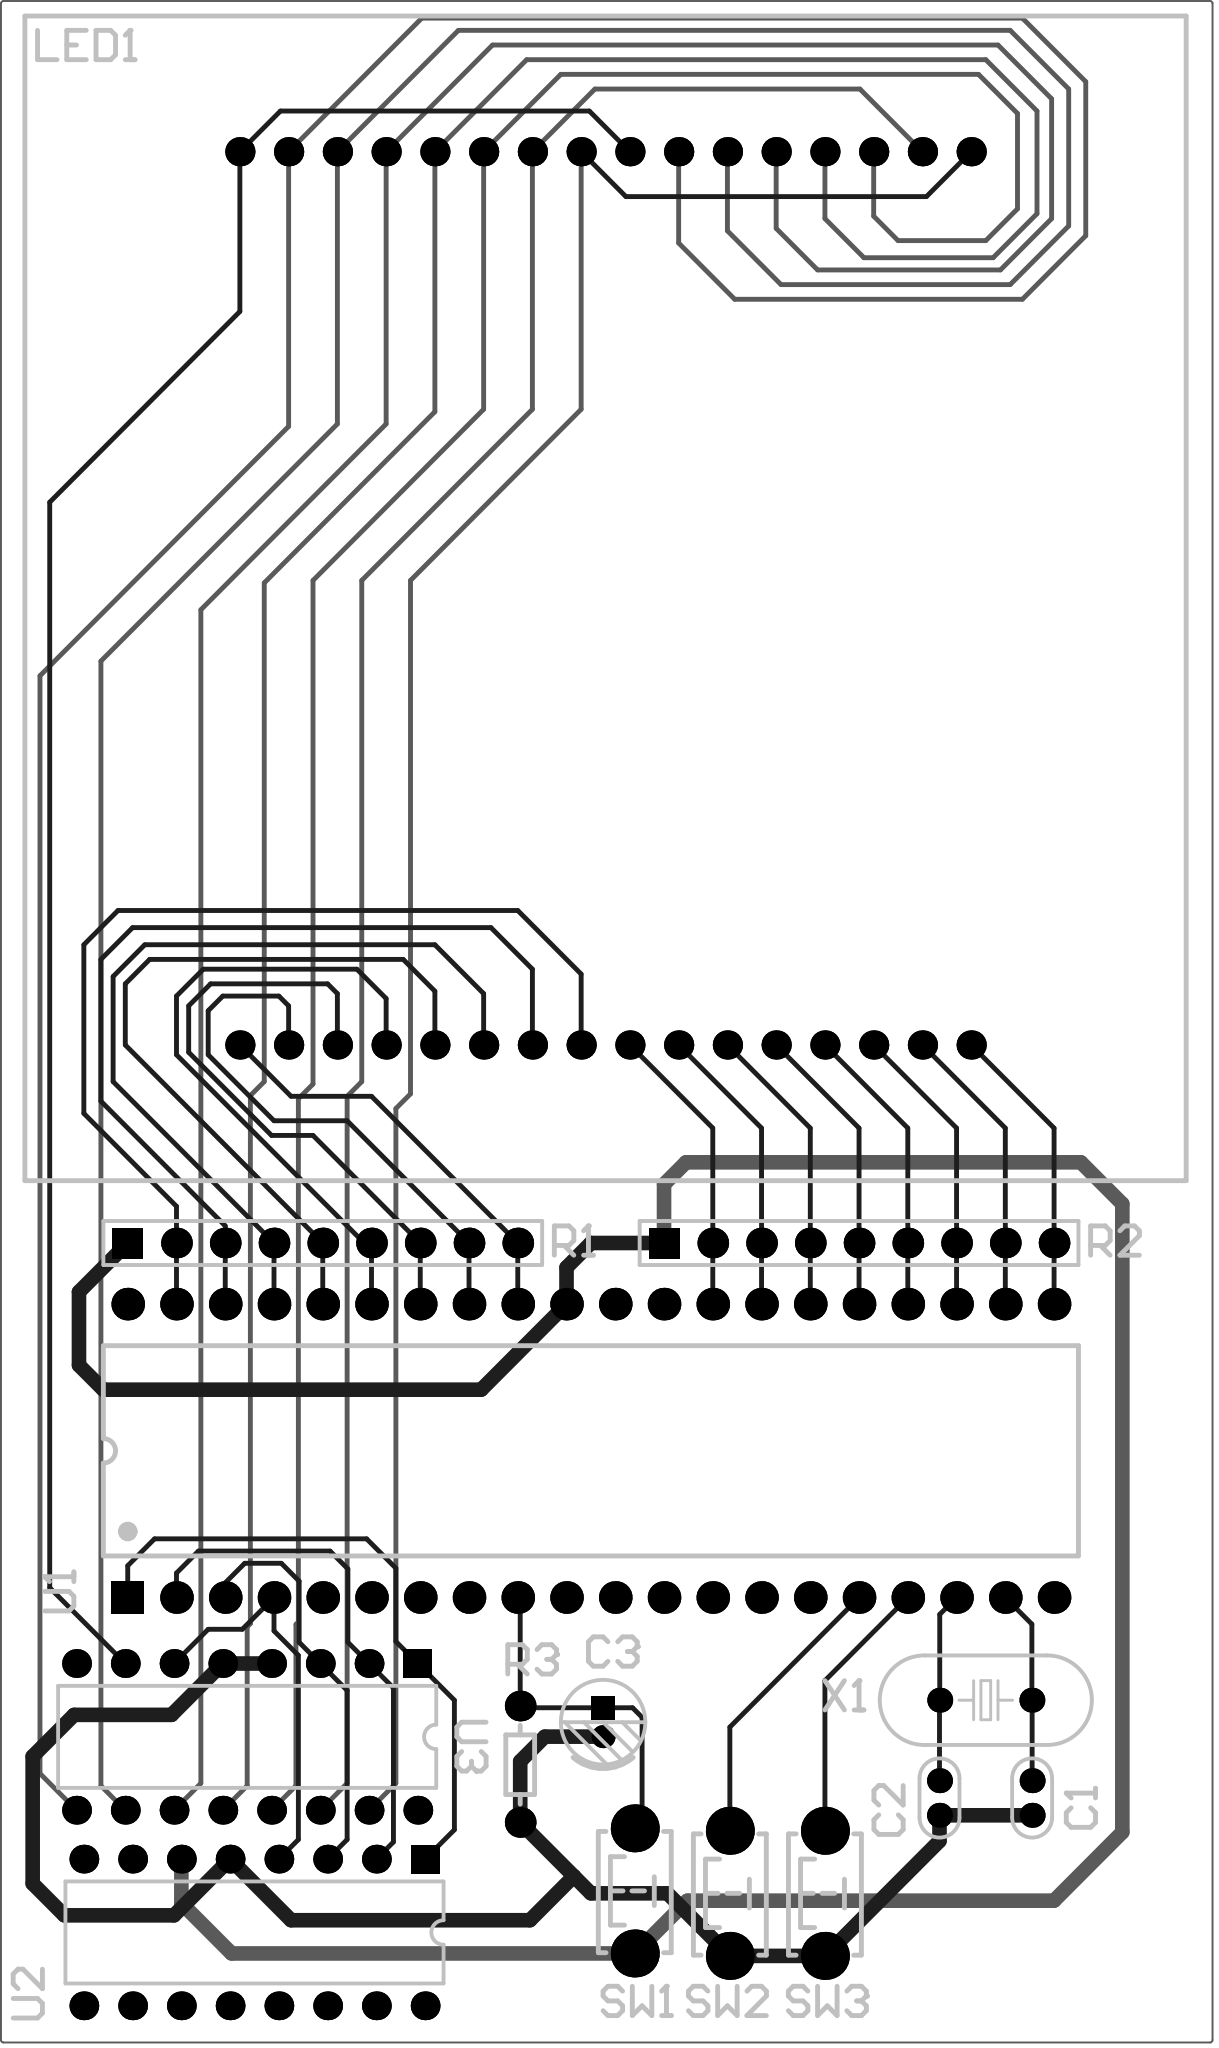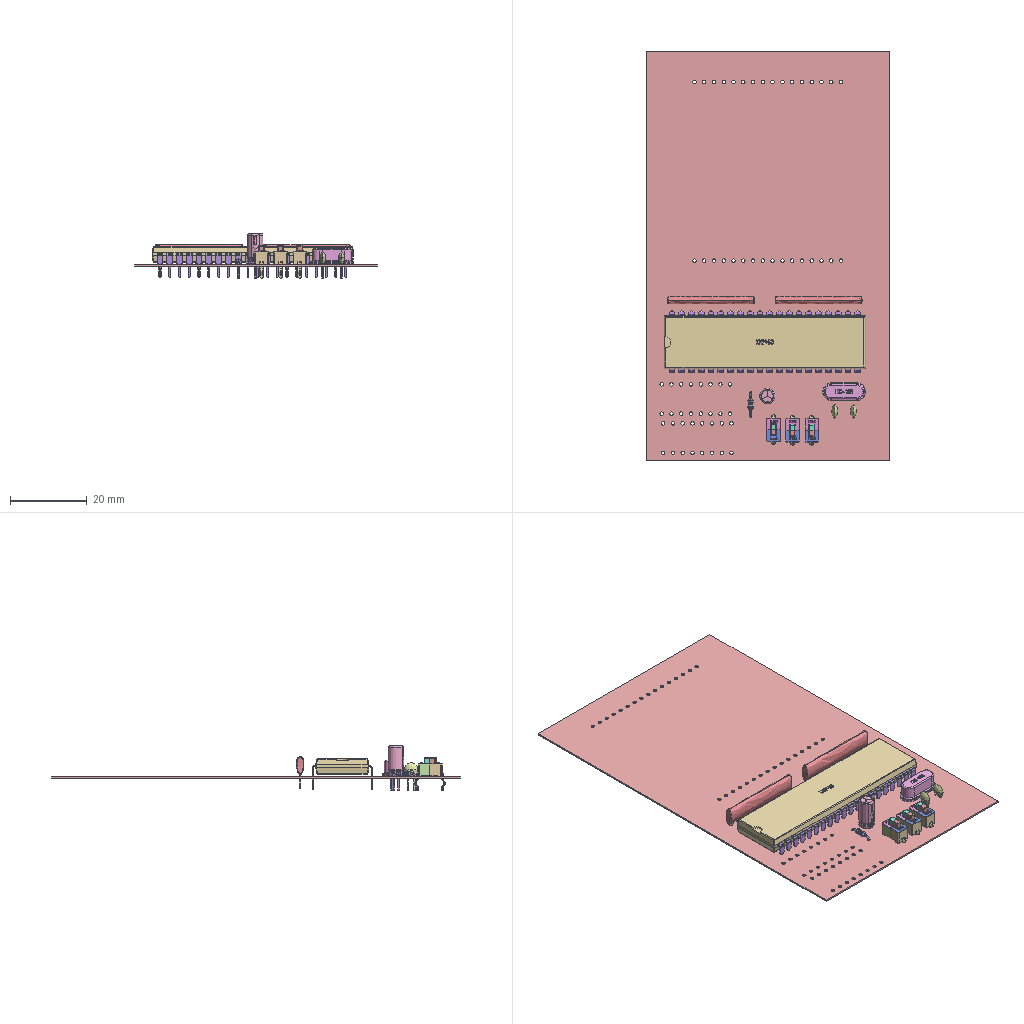Circuit board layout | Altium Designer | box 63.1 x 106 x 11.5 mm
Layer stack:
# Altium Designer layer stack of  (unit mm; dielectric type: 0 none, 1 core, 2 prepreg, 3 surface material)
index,name,kind,layer,copper_thickness_mm,dielectric_type,dielectric_thickness_mm,dielectric_material,dielectric_constant
0,Top Paste,other,,,,,,
1,Top Overlay,other,,,,,,
2,Top Solder,dielectric,,,3,0.0102,Solder Resist,3.5
3,Top Layer,copper,Top Layer,0.0356,,,,
4,Dielectric 1,dielectric,,,0,0.32,FR-4,4.8
5,Bottom Layer,copper,Bottom Layer,0.0356,,,,
6,Bottom Solder,dielectric,,,3,0.0102,Solder Resist,3.5
7,Bottom Overlay,other,,,,,,
8,Bottom Paste,other,,,,,,
# drill layer pairs: low layer,high layer
drill_pair,Top Layer,Bottom Layer
Part placement:
Designator,Comment,Layer,Footprint,Center-X(mm),Center-Y(mm),Rotation
X1,12MHz,TopLayer,OSC_HC-49S,143.891,35.687,360
U3,74HC138,TopLayer,648-08,105.41,33.782,180
U2,74HC138,TopLayer,648-08,105.791,23.622,180
U1,AT89C52,TopLayer,DIP40,123.317,48.641,90
SW3,3x6x5,TopLayer,TSW_DIP-3*6*5,135.509,25.654,90
SW2,3x6x5,TopLayer,TSW_DIP-3*6*5,130.556,25.654,90
SW1,3x6x5,TopLayer,TSW_DIP-3*6*5,125.603,25.781,90
R3,10K,TopLayer,RS_1/8W,119.634,32.361,90
R2,561,TopLayer,R_SIP9-2.54,137.287,59.436,360
R1,561,TopLayer,R_SIP9-2.54,109.347,59.436,360
LED1,RGB_Matrix_8x8,TopLayer,RGB_MATRIX_8X8,124.079,92.923,0
C3,10uF,TopLayer,CAP_1.5*4*8,123.952,34.544,270
C2,30pF,TopLayer,CC_1.8*3.6,141.478,30.607,90
C1,30pF,TopLayer,CC_1.8*3.6,146.304,30.607,90
Pad and via stacks:
# Altium Designer via and pad stacks of  (unit mm). Each distinct definition once, with the count of objects using it.
# via: kind,start_layer,end_layer,hole_mm,diameter_mm,mode(0 simple;1 top-mid-bottom;2 full stack),diameter_per_layer,count,example_net
# pad: kind,layer,hole_mm,hole_type(0 round;1 square;2 slot),plating,top_size,top_shape(1 round;2 rect;3 octagon;9 rounded rect),mid_size,bottom_size,mode,footprint,size_per_layer,count,example
pad,Multi-Layer,0.5,0,plated,1.3x1.3,1,1.3x1.3,1.3x1.3,0,CC 1.8*3.6,,4,C1.2
pad,Multi-Layer,1.2,0,plated,2.5x2.5,1,2.5x2.5,2.5x2.5,0,TSW DIP-3*6*5,,6,SW3.1
pad,Multi-Layer,0.9144,0,plated,1.524x1.524,1,1.524x1.524,1.524x1.524,0,RGB_MATRIX_8X8,,32,LED1.32
pad,Multi-Layer,0.7,0,plated,1.6x1.6,1,1.6x1.6,1.6x1.6,0,R SIP9-2.54,,16,R1.5
pad,Multi-Layer,0.7,0,plated,1.6x1.6,2,1.6x1.6,1.6x1.6,0,R SIP9-2.54,,2,R1.1
pad,Multi-Layer,0.8,0,plated,1.7x1.7,1,1.7x1.7,1.7x1.7,0,DIP40,,39,U1.21
pad,Multi-Layer,0.8,0,plated,1.7x1.7,2,1.7x1.7,1.7x1.7,0,DIP40,,1,U1.1
pad,Multi-Layer,0.6,0,plated,1.3x1.3,1,1.3x1.3,1.3x1.3,0,OSC HC-49S,,2,X1.2
pad,Multi-Layer,0.9,0,plated,1.5x1.5,2,1.5x1.5,1.5x1.5,0,648-08,,2,U2.1
pad,Multi-Layer,0.9,0,plated,1.5x1.5,1,1.5x1.5,1.5x1.5,0,648-08,,30,U2.2
pad,Multi-Layer,0.6,0,plated,1.2x1.2,1,1.2x1.2,1.2x1.2,0,CAP 1.5*4*8,,1,C3.2
pad,Multi-Layer,0.6,0,plated,1.2x1.2,2,1.2x1.2,1.2x1.2,0,CAP 1.5*4*8,,1,C3.1
pad,Multi-Layer,0.6,0,plated,1.6x1.6,1,1.6x1.6,1.6x1.6,0,RS 1/8W,,2,R3.1
Design rules, without the lines most boards share:
# Altium Designer design rules of  (exported by Altium Designer, unit mm)
# columns: name | kind | enabled | priority | scope1 | scope2 | descriptor | typed fields (field=value)
SilkToSilkClearance | 55 | enabled | 1 | All | All | Silk to Silk (Clearance=0mil) (All),(All) |
SilkToSolderMaskClearance | 54 | enabled | 1 | IsPad | All | Silk To Solder Mask (Clearance=0mil) (IsPad),(All) |
MinimumSolderMaskSliver | 53 | enabled | 1 | All | All | Minimum Solder Mask Sliver (Gap=0mil) (All),(All) |
HoleToHoleClearance | 52 | enabled | 1 | All | All | Hole To Hole Clearance (Gap=10mil) (All),(All) | gap=0.254
DiffPairsRouting | 51 | enabled | 1 | All | All | Differential Pairs Uncoupled Length using the Gap Constraints (Min=10mil) (Max=10mil) (Prefered=10mil)  and Width Constraints (Min=15mil) (Max=15mil) (Prefered=15mil) (All) |
SolderMaskExpansion | 13 | enabled | 1 | All | All | Solder Mask Expansion (Expansion =4mil) (All) | expansion=0.1016
PasteMaskExpansion | 14 | enabled | 1 | All | All | Paste Mask Expansion (Expansion =0mil) (All) | expansion=0
RoutingVias | 11 | enabled | 1 | All | All | Routing Via (MinHoleWidth=28mil) (MaxHoleWidth=28mil) (PreferredHoleWidth=28mil) (MinWidth=50mil) (MaxWidth=50mil) (PreferedWidth=50mil) (All) | via_min_hole=0.7112 via_max_hole=0.7112 via_preferred_diameter=1.27 via_preferred_hole=0.7112
Width | 2 | enabled | 1 | All | All | Width Constraint (Min=10mil) (Max=30mil) (Preferred=10mil) (All) |
PolygonConnect | 20 | enabled | 1 | All | All | Polygon Connect Rule(Relief Connect )(Conductor Width=10mil) (Relief Angle=90 Angle) (Entries=4) (Air Gap Width=10mil) (All),(All) | connect_style(0=relief,1=direct,2=none)=0 relief_conductor_width=0.254 relief_entries=4
PlaneConnect | 6 | enabled | 1 | All | All | Power Plane Connect Rule(Relief Connect )(Expansion=20mil) (Conductor Width=10mil) (Air Gap=10mil) (Entries=4) (All) | relief_conductor_width=0.254 relief_entries=4 relief_expansion=0.508
Clearance | 0 | enabled | 1 | All | All | Clearance Constraint (Gap=10mil) (All),(All) | gap=0.254
Classes set for this board:
# Altium Designer classes of  (member kind: 0 net, 1 component, 2 from-to, 3 pad, 4 layer, 5 differential pair, 6 design channel, 7 polygon, 8 structure, 9 xSignal)
# columns: class name | member kind | superclass | members
Sheet1(3) | 1 | no | C1; C2; C3; LED1; R1; R2; R3; SW1; SW2; SW3; U1; U2; U3; X1;